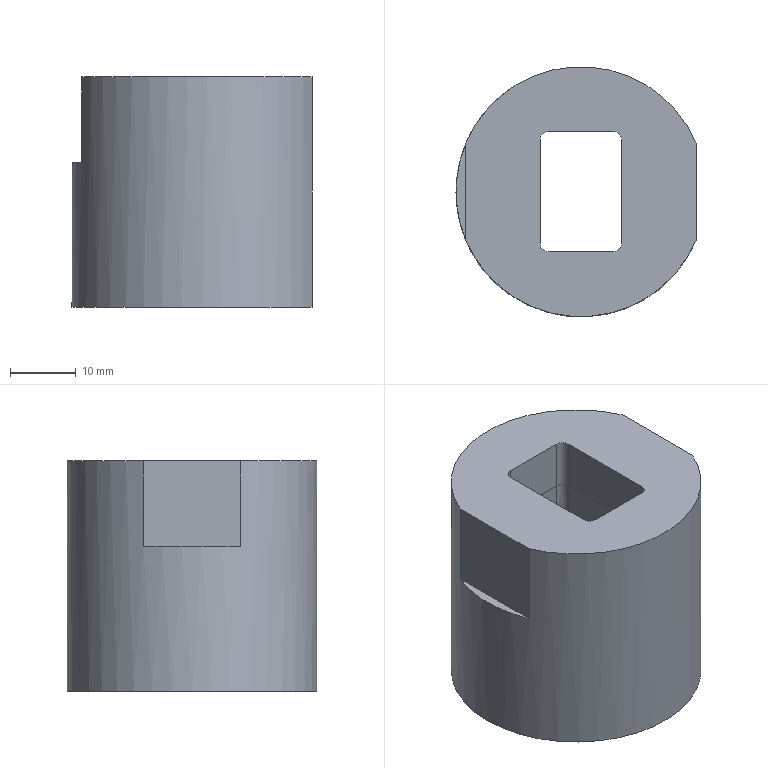Part | STEP file | lll_id4658_x_t | 1 solid | 22 faces | box 36.5 x 38 x 35 mm | volume 30517 mm3 | plane 13 | cylinder 5 | cone 4 | commonest cylinder face diameters 2.4 x4 38 x1
STEP:
#1=CARTESIAN_POINT('',(497.87,-357.252,-35.));
#2=VERTEX_POINT('',#1);
#3=CARTESIAN_POINT('',(487.87,-357.252,-35.));
#4=VERTEX_POINT('',#3);
#5=CARTESIAN_POINT('',(492.87,-357.252,-35.));
#6=DIRECTION('',(-1.,0.,0.));
#7=VECTOR('',#6,1.);
#8=LINE('',#5,#7);
#9=EDGE_CURVE('',#2,#4,#8,.T.);
#10=ORIENTED_EDGE('',*,*,#9,.F.);
#11=CARTESIAN_POINT('',(499.783,-355.34,-35.));
#12=VERTEX_POINT('',#11);
#13=CARTESIAN_POINT('',(497.87,-355.34,-35.));
#14=DIRECTION('',(0.,0.,-1.));
#15=DIRECTION('',(-1.,0.,0.));
#16=AXIS2_PLACEMENT_3D('',#13,#14,#15);
#17=CIRCLE('',#16,1.912);
#18=EDGE_CURVE('',#12,#2,#17,.T.);
#19=ORIENTED_EDGE('',*,*,#18,.F.);
#20=CARTESIAN_POINT('',(499.783,-339.5,-35.));
#21=VERTEX_POINT('',#20);
#22=CARTESIAN_POINT('',(499.783,-352.92,-35.));
#23=DIRECTION('',(0.,-1.,0.));
#24=VECTOR('',#23,1.);
#25=LINE('',#22,#24);
#26=EDGE_CURVE('',#21,#12,#25,.T.);
#27=ORIENTED_EDGE('',*,*,#26,.F.);
#28=CARTESIAN_POINT('',(497.87,-337.588,-35.));
#29=VERTEX_POINT('',#28);
#30=CARTESIAN_POINT('',(497.87,-339.5,-35.));
#31=DIRECTION('',(0.,0.,-1.));
#32=DIRECTION('',(-1.,0.,0.));
#33=AXIS2_PLACEMENT_3D('',#30,#31,#32);
#34=CIRCLE('',#33,1.912);
#35=EDGE_CURVE('',#29,#21,#34,.T.);
#36=ORIENTED_EDGE('',*,*,#35,.F.);
#37=CARTESIAN_POINT('',(487.87,-337.588,-35.));
#38=VERTEX_POINT('',#37);
#39=CARTESIAN_POINT('',(492.87,-337.588,-35.));
#40=DIRECTION('',(1.,0.,0.));
#41=VECTOR('',#40,1.);
#42=LINE('',#39,#41);
#43=EDGE_CURVE('',#38,#29,#42,.T.);
#44=ORIENTED_EDGE('',*,*,#43,.F.);
#45=CARTESIAN_POINT('',(485.958,-339.5,-35.));
#46=VERTEX_POINT('',#45);
#47=CARTESIAN_POINT('',(487.87,-339.5,-35.));
#48=DIRECTION('',(0.,0.,-1.));
#49=DIRECTION('',(-1.,0.,0.));
#50=AXIS2_PLACEMENT_3D('',#47,#48,#49);
#51=CIRCLE('',#50,1.912);
#52=EDGE_CURVE('',#46,#38,#51,.T.);
#53=ORIENTED_EDGE('',*,*,#52,.F.);
#54=CARTESIAN_POINT('',(485.958,-355.34,-35.));
#55=VERTEX_POINT('',#54);
#56=CARTESIAN_POINT('',(485.958,-352.92,-35.));
#57=DIRECTION('',(0.,1.,0.));
#58=VECTOR('',#57,1.);
#59=LINE('',#56,#58);
#60=EDGE_CURVE('',#55,#46,#59,.T.);
#61=ORIENTED_EDGE('',*,*,#60,.F.);
#62=CARTESIAN_POINT('',(487.87,-355.34,-35.));
#63=DIRECTION('',(0.,0.,-1.));
#64=DIRECTION('',(-1.,0.,0.));
#65=AXIS2_PLACEMENT_3D('',#62,#63,#64);
#66=CIRCLE('',#65,1.912);
#67=EDGE_CURVE('',#4,#55,#66,.T.);
#68=ORIENTED_EDGE('',*,*,#67,.F.);
#69=EDGE_LOOP('',(#10,#19,#27,#36,#44,#53,#61,#68));
#70=FACE_BOUND('',#69,.T.);
#71=CARTESIAN_POINT('',(510.37,-340.021,-35.));
#72=VERTEX_POINT('',#71);
#73=CARTESIAN_POINT('',(510.37,-354.819,-35.));
#74=VERTEX_POINT('',#73);
#75=CARTESIAN_POINT('',(510.37,-340.919,-35.));
#76=DIRECTION('',(0.,-1.,0.));
#77=VECTOR('',#76,1.);
#78=LINE('',#75,#77);
#79=EDGE_CURVE('',#72,#74,#78,.T.);
#80=ORIENTED_EDGE('',*,*,#79,.T.);
#81=CARTESIAN_POINT('',(492.87,-347.42,-35.));
#82=DIRECTION('',(0.,0.,1.));
#83=DIRECTION('',(1.,0.,0.));
#84=AXIS2_PLACEMENT_3D('',#81,#82,#83);
#85=CIRCLE('',#84,19.);
#86=EDGE_CURVE('',#72,#74,#85,.T.);
#87=ORIENTED_EDGE('',*,*,#86,.F.);
#88=EDGE_LOOP('',(#80,#87));
#89=FACE_BOUND('',#88,.T.);
#90=CARTESIAN_POINT('',(492.87,-352.92,-35.));
#91=DIRECTION('',(0.,0.,-1.));
#92=DIRECTION('',(0.,1.,0.));
#93=AXIS2_PLACEMENT_3D('',#90,#91,#92);
#94=PLANE('',#93);
#95=ADVANCED_FACE('',(#70,#89),#94,.T.);
#96=CARTESIAN_POINT('',(475.37,-340.021,0.));
#97=VERTEX_POINT('',#96);
#98=CARTESIAN_POINT('',(475.37,-340.021,-13.));
#99=VERTEX_POINT('',#98);
#100=CARTESIAN_POINT('',(475.37,-340.021,-15.));
#101=DIRECTION('',(0.,0.,-1.));
#102=VECTOR('',#101,1.);
#103=LINE('',#100,#102);
#104=EDGE_CURVE('',#97,#99,#103,.T.);
#105=ORIENTED_EDGE('',*,*,#104,.F.);
#106=CARTESIAN_POINT('',(510.37,-340.021,0.));
#107=VERTEX_POINT('',#106);
#108=CARTESIAN_POINT('',(492.87,-347.42,0.));
#109=DIRECTION('',(0.,0.,1.));
#110=DIRECTION('',(1.,0.,0.));
#111=AXIS2_PLACEMENT_3D('',#108,#109,#110);
#112=CIRCLE('',#111,19.);
#113=EDGE_CURVE('',#107,#97,#112,.T.);
#114=ORIENTED_EDGE('',*,*,#113,.F.);
#115=CARTESIAN_POINT('',(510.37,-340.021,0.));
#116=DIRECTION('',(0.,0.,-1.));
#117=VECTOR('',#116,1.);
#118=LINE('',#115,#117);
#119=EDGE_CURVE('',#107,#72,#118,.T.);
#120=ORIENTED_EDGE('',*,*,#119,.T.);
#121=ORIENTED_EDGE('',*,*,#86,.T.);
#122=CARTESIAN_POINT('',(510.37,-354.819,0.));
#123=VERTEX_POINT('',#122);
#124=CARTESIAN_POINT('',(510.37,-354.819,-15.));
#125=DIRECTION('',(0.,0.,1.));
#126=VECTOR('',#125,1.);
#127=LINE('',#124,#126);
#128=EDGE_CURVE('',#74,#123,#127,.T.);
#129=ORIENTED_EDGE('',*,*,#128,.T.);
#130=CARTESIAN_POINT('',(475.37,-354.819,0.));
#131=VERTEX_POINT('',#130);
#132=CARTESIAN_POINT('',(492.87,-347.42,0.));
#133=DIRECTION('',(0.,0.,1.));
#134=DIRECTION('',(1.,0.,0.));
#135=AXIS2_PLACEMENT_3D('',#132,#133,#134);
#136=CIRCLE('',#135,19.);
#137=EDGE_CURVE('',#131,#123,#136,.T.);
#138=ORIENTED_EDGE('',*,*,#137,.F.);
#139=CARTESIAN_POINT('',(475.37,-354.819,-13.));
#140=VERTEX_POINT('',#139);
#141=CARTESIAN_POINT('',(475.37,-354.819,-15.));
#142=DIRECTION('',(0.,0.,1.));
#143=VECTOR('',#142,1.);
#144=LINE('',#141,#143);
#145=EDGE_CURVE('',#140,#131,#144,.T.);
#146=ORIENTED_EDGE('',*,*,#145,.F.);
#147=CARTESIAN_POINT('',(492.87,-347.42,-13.));
#148=DIRECTION('',(0.,0.,1.));
#149=DIRECTION('',(1.,0.,0.));
#150=AXIS2_PLACEMENT_3D('',#147,#148,#149);
#151=CIRCLE('',#150,19.);
#152=EDGE_CURVE('',#99,#140,#151,.T.);
#153=ORIENTED_EDGE('',*,*,#152,.F.);
#154=EDGE_LOOP('',(#105,#114,#120,#121,#129,#138,#146,#153));
#155=FACE_OUTER_BOUND('',#154,.T.);
#156=CARTESIAN_POINT('',(492.87,-347.42,-15.));
#157=DIRECTION('',(0.,0.,-1.));
#158=DIRECTION('',(0.,-1.,0.));
#159=AXIS2_PLACEMENT_3D('',#156,#157,#158);
#160=CYLINDRICAL_SURFACE('',#159,19.);
#161=ADVANCED_FACE('',(#155),#160,.T.);
#162=CARTESIAN_POINT('',(475.37,-347.42,0.));
#163=DIRECTION('',(0.,1.,0.));
#164=VECTOR('',#163,1.);
#165=LINE('',#162,#164);
#166=EDGE_CURVE('',#131,#97,#165,.T.);
#167=ORIENTED_EDGE('',*,*,#166,.F.);
#168=ORIENTED_EDGE('',*,*,#137,.T.);
#169=CARTESIAN_POINT('',(510.37,-340.919,0.));
#170=DIRECTION('',(0.,1.,0.));
#171=VECTOR('',#170,1.);
#172=LINE('',#169,#171);
#173=EDGE_CURVE('',#123,#107,#172,.T.);
#174=ORIENTED_EDGE('',*,*,#173,.T.);
#175=ORIENTED_EDGE('',*,*,#113,.T.);
#176=EDGE_LOOP('',(#167,#168,#174,#175));
#177=FACE_BOUND('',#176,.T.);
#178=CARTESIAN_POINT('',(487.87,-356.54,0.));
#179=VERTEX_POINT('',#178);
#180=CARTESIAN_POINT('',(486.67,-355.34,0.));
#181=VERTEX_POINT('',#180);
#182=CARTESIAN_POINT('',(487.87,-355.34,0.));
#183=DIRECTION('',(0.,0.,-1.));
#184=DIRECTION('',(1.,0.,0.));
#185=AXIS2_PLACEMENT_3D('',#182,#183,#184);
#186=CIRCLE('',#185,1.2);
#187=EDGE_CURVE('',#179,#181,#186,.T.);
#188=ORIENTED_EDGE('',*,*,#187,.T.);
#189=CARTESIAN_POINT('',(486.67,-339.5,0.));
#190=VERTEX_POINT('',#189);
#191=CARTESIAN_POINT('',(486.67,-347.42,0.));
#192=DIRECTION('',(0.,1.,0.));
#193=VECTOR('',#192,1.);
#194=LINE('',#191,#193);
#195=EDGE_CURVE('',#181,#190,#194,.T.);
#196=ORIENTED_EDGE('',*,*,#195,.T.);
#197=CARTESIAN_POINT('',(487.87,-338.3,0.));
#198=VERTEX_POINT('',#197);
#199=CARTESIAN_POINT('',(487.87,-339.5,0.));
#200=DIRECTION('',(0.,0.,-1.));
#201=DIRECTION('',(1.,0.,0.));
#202=AXIS2_PLACEMENT_3D('',#199,#200,#201);
#203=CIRCLE('',#202,1.2);
#204=EDGE_CURVE('',#190,#198,#203,.T.);
#205=ORIENTED_EDGE('',*,*,#204,.T.);
#206=CARTESIAN_POINT('',(497.87,-338.3,0.));
#207=VERTEX_POINT('',#206);
#208=CARTESIAN_POINT('',(492.87,-338.3,0.));
#209=DIRECTION('',(1.,0.,0.));
#210=VECTOR('',#209,1.);
#211=LINE('',#208,#210);
#212=EDGE_CURVE('',#198,#207,#211,.T.);
#213=ORIENTED_EDGE('',*,*,#212,.T.);
#214=CARTESIAN_POINT('',(499.07,-339.5,0.));
#215=VERTEX_POINT('',#214);
#216=CARTESIAN_POINT('',(497.87,-339.5,0.));
#217=DIRECTION('',(0.,0.,-1.));
#218=DIRECTION('',(1.,0.,0.));
#219=AXIS2_PLACEMENT_3D('',#216,#217,#218);
#220=CIRCLE('',#219,1.2);
#221=EDGE_CURVE('',#207,#215,#220,.T.);
#222=ORIENTED_EDGE('',*,*,#221,.T.);
#223=CARTESIAN_POINT('',(499.07,-355.34,0.));
#224=VERTEX_POINT('',#223);
#225=CARTESIAN_POINT('',(499.07,-347.42,0.));
#226=DIRECTION('',(0.,-1.,0.));
#227=VECTOR('',#226,1.);
#228=LINE('',#225,#227);
#229=EDGE_CURVE('',#215,#224,#228,.T.);
#230=ORIENTED_EDGE('',*,*,#229,.T.);
#231=CARTESIAN_POINT('',(497.87,-356.54,0.));
#232=VERTEX_POINT('',#231);
#233=CARTESIAN_POINT('',(497.87,-355.34,0.));
#234=DIRECTION('',(0.,0.,-1.));
#235=DIRECTION('',(1.,0.,0.));
#236=AXIS2_PLACEMENT_3D('',#233,#234,#235);
#237=CIRCLE('',#236,1.2);
#238=EDGE_CURVE('',#224,#232,#237,.T.);
#239=ORIENTED_EDGE('',*,*,#238,.T.);
#240=CARTESIAN_POINT('',(492.87,-356.54,0.));
#241=DIRECTION('',(-1.,0.,0.));
#242=VECTOR('',#241,1.);
#243=LINE('',#240,#242);
#244=EDGE_CURVE('',#232,#179,#243,.T.);
#245=ORIENTED_EDGE('',*,*,#244,.T.);
#246=EDGE_LOOP('',(#188,#196,#205,#213,#222,#230,#239,#245));
#247=FACE_BOUND('',#246,.T.);
#248=CARTESIAN_POINT('',(492.87,-347.42,0.));
#249=DIRECTION('',(0.,0.,1.));
#250=DIRECTION('',(-1.,0.,0.));
#251=AXIS2_PLACEMENT_3D('',#248,#249,#250);
#252=PLANE('',#251);
#253=ADVANCED_FACE('',(#177,#247),#252,.T.);
#254=ORIENTED_EDGE('',*,*,#79,.F.);
#255=ORIENTED_EDGE('',*,*,#119,.F.);
#256=ORIENTED_EDGE('',*,*,#173,.F.);
#257=ORIENTED_EDGE('',*,*,#128,.F.);
#258=EDGE_LOOP('',(#254,#255,#256,#257));
#259=FACE_OUTER_BOUND('',#258,.T.);
#260=CARTESIAN_POINT('',(510.37,-340.919,0.));
#261=DIRECTION('',(-1.,0.,0.));
#262=DIRECTION('',(0.,0.,1.));
#263=AXIS2_PLACEMENT_3D('',#260,#261,#262);
#264=PLANE('',#263);
#265=ADVANCED_FACE('',(#259),#264,.F.);
#266=CARTESIAN_POINT('',(487.87,-356.54,-7.8));
#267=VERTEX_POINT('',#266);
#268=CARTESIAN_POINT('',(487.87,-356.54,2.5));
#269=DIRECTION('',(0.,0.,1.));
#270=VECTOR('',#269,1.);
#271=LINE('',#268,#270);
#272=EDGE_CURVE('',#267,#179,#271,.T.);
#273=ORIENTED_EDGE('',*,*,#272,.F.);
#274=CARTESIAN_POINT('',(486.67,-355.34,-7.8));
#275=VERTEX_POINT('',#274);
#276=CARTESIAN_POINT('',(487.87,-355.34,-7.8));
#277=DIRECTION('',(0.,0.,1.));
#278=DIRECTION('',(1.,0.,0.));
#279=AXIS2_PLACEMENT_3D('',#276,#277,#278);
#280=CIRCLE('',#279,1.2);
#281=EDGE_CURVE('',#275,#267,#280,.T.);
#282=ORIENTED_EDGE('',*,*,#281,.F.);
#283=CARTESIAN_POINT('',(486.67,-355.34,2.5));
#284=DIRECTION('',(0.,0.,1.));
#285=VECTOR('',#284,1.);
#286=LINE('',#283,#285);
#287=EDGE_CURVE('',#275,#181,#286,.T.);
#288=ORIENTED_EDGE('',*,*,#287,.T.);
#289=ORIENTED_EDGE('',*,*,#187,.F.);
#290=EDGE_LOOP('',(#273,#282,#288,#289));
#291=FACE_OUTER_BOUND('',#290,.T.);
#292=CARTESIAN_POINT('',(487.87,-355.34,2.5));
#293=DIRECTION('',(0.,0.,-1.));
#294=DIRECTION('',(-1.,0.,0.));
#295=AXIS2_PLACEMENT_3D('',#292,#293,#294);
#296=CYLINDRICAL_SURFACE('',#295,1.2);
#297=ADVANCED_FACE('',(#291),#296,.F.);
#298=CARTESIAN_POINT('',(497.87,-356.54,-7.8));
#299=VERTEX_POINT('',#298);
#300=CARTESIAN_POINT('',(497.87,-356.54,2.5));
#301=DIRECTION('',(0.,0.,1.));
#302=VECTOR('',#301,1.);
#303=LINE('',#300,#302);
#304=EDGE_CURVE('',#299,#232,#303,.T.);
#305=ORIENTED_EDGE('',*,*,#304,.F.);
#306=CARTESIAN_POINT('',(487.87,-356.54,-7.8));
#307=DIRECTION('',(1.,0.,0.));
#308=VECTOR('',#307,1.);
#309=LINE('',#306,#308);
#310=EDGE_CURVE('',#267,#299,#309,.T.);
#311=ORIENTED_EDGE('',*,*,#310,.F.);
#312=ORIENTED_EDGE('',*,*,#272,.T.);
#313=ORIENTED_EDGE('',*,*,#244,.F.);
#314=EDGE_LOOP('',(#305,#311,#312,#313));
#315=FACE_OUTER_BOUND('',#314,.T.);
#316=CARTESIAN_POINT('',(487.87,-356.54,2.5));
#317=DIRECTION('',(0.,-1.,0.));
#318=DIRECTION('',(0.,0.,1.));
#319=AXIS2_PLACEMENT_3D('',#316,#317,#318);
#320=PLANE('',#319);
#321=ADVANCED_FACE('',(#315),#320,.F.);
#322=CARTESIAN_POINT('',(499.07,-355.34,-7.8));
#323=VERTEX_POINT('',#322);
#324=CARTESIAN_POINT('',(499.07,-355.34,2.5));
#325=DIRECTION('',(0.,0.,1.));
#326=VECTOR('',#325,1.);
#327=LINE('',#324,#326);
#328=EDGE_CURVE('',#323,#224,#327,.T.);
#329=ORIENTED_EDGE('',*,*,#328,.F.);
#330=CARTESIAN_POINT('',(497.87,-355.34,-7.8));
#331=DIRECTION('',(0.,0.,1.));
#332=DIRECTION('',(1.,0.,0.));
#333=AXIS2_PLACEMENT_3D('',#330,#331,#332);
#334=CIRCLE('',#333,1.2);
#335=EDGE_CURVE('',#299,#323,#334,.T.);
#336=ORIENTED_EDGE('',*,*,#335,.F.);
#337=ORIENTED_EDGE('',*,*,#304,.T.);
#338=ORIENTED_EDGE('',*,*,#238,.F.);
#339=EDGE_LOOP('',(#329,#336,#337,#338));
#340=FACE_OUTER_BOUND('',#339,.T.);
#341=CARTESIAN_POINT('',(497.87,-355.34,2.5));
#342=DIRECTION('',(0.,0.,-1.));
#343=DIRECTION('',(-1.,0.,0.));
#344=AXIS2_PLACEMENT_3D('',#341,#342,#343);
#345=CYLINDRICAL_SURFACE('',#344,1.2);
#346=ADVANCED_FACE('',(#340),#345,.F.);
#347=CARTESIAN_POINT('',(499.07,-339.5,-7.8));
#348=VERTEX_POINT('',#347);
#349=CARTESIAN_POINT('',(499.07,-339.5,2.5));
#350=DIRECTION('',(0.,0.,1.));
#351=VECTOR('',#350,1.);
#352=LINE('',#349,#351);
#353=EDGE_CURVE('',#348,#215,#352,.T.);
#354=ORIENTED_EDGE('',*,*,#353,.F.);
#355=CARTESIAN_POINT('',(499.07,-355.34,-7.8));
#356=DIRECTION('',(0.,1.,0.));
#357=VECTOR('',#356,1.);
#358=LINE('',#355,#357);
#359=EDGE_CURVE('',#323,#348,#358,.T.);
#360=ORIENTED_EDGE('',*,*,#359,.F.);
#361=ORIENTED_EDGE('',*,*,#328,.T.);
#362=ORIENTED_EDGE('',*,*,#229,.F.);
#363=EDGE_LOOP('',(#354,#360,#361,#362));
#364=FACE_OUTER_BOUND('',#363,.T.);
#365=CARTESIAN_POINT('',(499.07,-355.42,2.5));
#366=DIRECTION('',(1.,0.,0.));
#367=DIRECTION('',(0.,0.,-1.));
#368=AXIS2_PLACEMENT_3D('',#365,#366,#367);
#369=PLANE('',#368);
#370=ADVANCED_FACE('',(#364),#369,.F.);
#371=CARTESIAN_POINT('',(497.87,-338.3,-7.8));
#372=VERTEX_POINT('',#371);
#373=CARTESIAN_POINT('',(497.87,-338.3,2.5));
#374=DIRECTION('',(0.,0.,1.));
#375=VECTOR('',#374,1.);
#376=LINE('',#373,#375);
#377=EDGE_CURVE('',#372,#207,#376,.T.);
#378=ORIENTED_EDGE('',*,*,#377,.F.);
#379=CARTESIAN_POINT('',(497.87,-339.5,-7.8));
#380=DIRECTION('',(0.,0.,1.));
#381=DIRECTION('',(1.,0.,0.));
#382=AXIS2_PLACEMENT_3D('',#379,#380,#381);
#383=CIRCLE('',#382,1.2);
#384=EDGE_CURVE('',#348,#372,#383,.T.);
#385=ORIENTED_EDGE('',*,*,#384,.F.);
#386=ORIENTED_EDGE('',*,*,#353,.T.);
#387=ORIENTED_EDGE('',*,*,#221,.F.);
#388=EDGE_LOOP('',(#378,#385,#386,#387));
#389=FACE_OUTER_BOUND('',#388,.T.);
#390=CARTESIAN_POINT('',(497.87,-339.5,2.5));
#391=DIRECTION('',(0.,0.,-1.));
#392=DIRECTION('',(-1.,0.,0.));
#393=AXIS2_PLACEMENT_3D('',#390,#391,#392);
#394=CYLINDRICAL_SURFACE('',#393,1.2);
#395=ADVANCED_FACE('',(#389),#394,.F.);
#396=CARTESIAN_POINT('',(487.87,-338.3,-7.8));
#397=VERTEX_POINT('',#396);
#398=CARTESIAN_POINT('',(487.87,-338.3,2.5));
#399=DIRECTION('',(0.,0.,1.));
#400=VECTOR('',#399,1.);
#401=LINE('',#398,#400);
#402=EDGE_CURVE('',#397,#198,#401,.T.);
#403=ORIENTED_EDGE('',*,*,#402,.F.);
#404=CARTESIAN_POINT('',(497.87,-338.3,-7.8));
#405=DIRECTION('',(-1.,0.,0.));
#406=VECTOR('',#405,1.);
#407=LINE('',#404,#406);
#408=EDGE_CURVE('',#372,#397,#407,.T.);
#409=ORIENTED_EDGE('',*,*,#408,.F.);
#410=ORIENTED_EDGE('',*,*,#377,.T.);
#411=ORIENTED_EDGE('',*,*,#212,.F.);
#412=EDGE_LOOP('',(#403,#409,#410,#411));
#413=FACE_OUTER_BOUND('',#412,.T.);
#414=CARTESIAN_POINT('',(497.87,-338.3,2.5));
#415=DIRECTION('',(0.,1.,0.));
#416=DIRECTION('',(0.,0.,-1.));
#417=AXIS2_PLACEMENT_3D('',#414,#415,#416);
#418=PLANE('',#417);
#419=ADVANCED_FACE('',(#413),#418,.F.);
#420=CARTESIAN_POINT('',(486.67,-339.5,-7.8));
#421=VERTEX_POINT('',#420);
#422=CARTESIAN_POINT('',(486.67,-339.5,2.5));
#423=DIRECTION('',(0.,0.,1.));
#424=VECTOR('',#423,1.);
#425=LINE('',#422,#424);
#426=EDGE_CURVE('',#421,#190,#425,.T.);
#427=ORIENTED_EDGE('',*,*,#426,.F.);
#428=CARTESIAN_POINT('',(487.87,-339.5,-7.8));
#429=DIRECTION('',(0.,0.,1.));
#430=DIRECTION('',(1.,0.,0.));
#431=AXIS2_PLACEMENT_3D('',#428,#429,#430);
#432=CIRCLE('',#431,1.2);
#433=EDGE_CURVE('',#397,#421,#432,.T.);
#434=ORIENTED_EDGE('',*,*,#433,.F.);
#435=ORIENTED_EDGE('',*,*,#402,.T.);
#436=ORIENTED_EDGE('',*,*,#204,.F.);
#437=EDGE_LOOP('',(#427,#434,#435,#436));
#438=FACE_OUTER_BOUND('',#437,.T.);
#439=CARTESIAN_POINT('',(487.87,-339.5,2.5));
#440=DIRECTION('',(0.,0.,-1.));
#441=DIRECTION('',(-1.,0.,0.));
#442=AXIS2_PLACEMENT_3D('',#439,#440,#441);
#443=CYLINDRICAL_SURFACE('',#442,1.2);
#444=ADVANCED_FACE('',(#438),#443,.F.);
#445=ORIENTED_EDGE('',*,*,#287,.F.);
#446=CARTESIAN_POINT('',(486.67,-339.5,-7.8));
#447=DIRECTION('',(0.,-1.,0.));
#448=VECTOR('',#447,1.);
#449=LINE('',#446,#448);
#450=EDGE_CURVE('',#421,#275,#449,.T.);
#451=ORIENTED_EDGE('',*,*,#450,.F.);
#452=ORIENTED_EDGE('',*,*,#426,.T.);
#453=ORIENTED_EDGE('',*,*,#195,.F.);
#454=EDGE_LOOP('',(#445,#451,#452,#453));
#455=FACE_OUTER_BOUND('',#454,.T.);
#456=CARTESIAN_POINT('',(486.67,-339.42,2.5));
#457=DIRECTION('',(-1.,0.,0.));
#458=DIRECTION('',(0.,0.,1.));
#459=AXIS2_PLACEMENT_3D('',#456,#457,#458);
#460=PLANE('',#459);
#461=ADVANCED_FACE('',(#455),#460,.F.);
#462=ORIENTED_EDGE('',*,*,#104,.T.);
#463=CARTESIAN_POINT('',(475.37,-347.42,-13.));
#464=DIRECTION('',(0.,-1.,0.));
#465=VECTOR('',#464,1.);
#466=LINE('',#463,#465);
#467=EDGE_CURVE('',#99,#140,#466,.T.);
#468=ORIENTED_EDGE('',*,*,#467,.T.);
#469=ORIENTED_EDGE('',*,*,#145,.T.);
#470=ORIENTED_EDGE('',*,*,#166,.T.);
#471=EDGE_LOOP('',(#462,#468,#469,#470));
#472=FACE_OUTER_BOUND('',#471,.T.);
#473=CARTESIAN_POINT('',(475.37,-347.42,-17.5));
#474=DIRECTION('',(1.,0.,0.));
#475=DIRECTION('',(0.,0.,-1.));
#476=AXIS2_PLACEMENT_3D('',#473,#474,#475);
#477=PLANE('',#476);
#478=ADVANCED_FACE('',(#472),#477,.F.);
#479=ORIENTED_EDGE('',*,*,#152,.T.);
#480=ORIENTED_EDGE('',*,*,#467,.F.);
#481=EDGE_LOOP('',(#479,#480));
#482=FACE_OUTER_BOUND('',#481,.T.);
#483=CARTESIAN_POINT('',(492.87,-347.42,-13.));
#484=DIRECTION('',(0.,0.,1.));
#485=DIRECTION('',(-1.,0.,0.));
#486=AXIS2_PLACEMENT_3D('',#483,#484,#485);
#487=PLANE('',#486);
#488=ADVANCED_FACE('',(#482),#487,.T.);
#489=ORIENTED_EDGE('',*,*,#9,.T.);
#490=CARTESIAN_POINT('',(487.87,-356.54,-7.8));
#491=DIRECTION('',(0.,-0.02618,-0.9997));
#492=VECTOR('',#491,1.);
#493=LINE('',#490,#492);
#494=EDGE_CURVE('',#267,#4,#493,.T.);
#495=ORIENTED_EDGE('',*,*,#494,.F.);
#496=ORIENTED_EDGE('',*,*,#310,.T.);
#497=CARTESIAN_POINT('',(497.87,-356.54,-7.8));
#498=DIRECTION('',(0.,-0.02618,-0.9997));
#499=VECTOR('',#498,1.);
#500=LINE('',#497,#499);
#501=EDGE_CURVE('',#299,#2,#500,.T.);
#502=ORIENTED_EDGE('',*,*,#501,.T.);
#503=EDGE_LOOP('',(#489,#495,#496,#502));
#504=FACE_OUTER_BOUND('',#503,.T.);
#505=CARTESIAN_POINT('',(487.87,-356.54,-7.8));
#506=DIRECTION('',(0.,0.9997,-0.02618));
#507=DIRECTION('',(0.,0.02618,0.9997));
#508=AXIS2_PLACEMENT_3D('',#505,#506,#507);
#509=PLANE('',#508);
#510=ADVANCED_FACE('',(#504),#509,.T.);
#511=ORIENTED_EDGE('',*,*,#18,.T.);
#512=ORIENTED_EDGE('',*,*,#501,.F.);
#513=ORIENTED_EDGE('',*,*,#335,.T.);
#514=CARTESIAN_POINT('',(499.07,-355.34,-7.8));
#515=DIRECTION('',(0.02618,-0.000000105,-0.9997));
#516=VECTOR('',#515,1.);
#517=LINE('',#514,#516);
#518=EDGE_CURVE('',#323,#12,#517,.T.);
#519=ORIENTED_EDGE('',*,*,#518,.T.);
#520=EDGE_LOOP('',(#511,#512,#513,#519));
#521=FACE_OUTER_BOUND('',#520,.T.);
#522=CARTESIAN_POINT('',(497.87,-355.34,-7.8));
#523=DIRECTION('',(0.,0.,-1.));
#524=DIRECTION('',(1.,0.,0.));
#525=AXIS2_PLACEMENT_3D('',#522,#523,#524);
#526=CONICAL_SURFACE('',#525,1.2,1.5);
#527=ADVANCED_FACE('',(#521),#526,.F.);
#528=ORIENTED_EDGE('',*,*,#26,.T.);
#529=ORIENTED_EDGE('',*,*,#518,.F.);
#530=ORIENTED_EDGE('',*,*,#359,.T.);
#531=CARTESIAN_POINT('',(499.07,-339.5,-7.8));
#532=DIRECTION('',(0.02618,0.,-0.9997));
#533=VECTOR('',#532,1.);
#534=LINE('',#531,#533);
#535=EDGE_CURVE('',#348,#21,#534,.T.);
#536=ORIENTED_EDGE('',*,*,#535,.T.);
#537=EDGE_LOOP('',(#528,#529,#530,#536));
#538=FACE_OUTER_BOUND('',#537,.T.);
#539=CARTESIAN_POINT('',(499.07,-355.34,-7.8));
#540=DIRECTION('',(-0.9997,0.,-0.02618));
#541=DIRECTION('',(-0.02618,0.,0.9997));
#542=AXIS2_PLACEMENT_3D('',#539,#540,#541);
#543=PLANE('',#542);
#544=ADVANCED_FACE('',(#538),#543,.T.);
#545=ORIENTED_EDGE('',*,*,#35,.T.);
#546=ORIENTED_EDGE('',*,*,#535,.F.);
#547=ORIENTED_EDGE('',*,*,#384,.T.);
#548=CARTESIAN_POINT('',(497.87,-338.3,-7.8));
#549=DIRECTION('',(0.,0.02618,-0.9997));
#550=VECTOR('',#549,1.);
#551=LINE('',#548,#550);
#552=EDGE_CURVE('',#372,#29,#551,.T.);
#553=ORIENTED_EDGE('',*,*,#552,.T.);
#554=EDGE_LOOP('',(#545,#546,#547,#553));
#555=FACE_OUTER_BOUND('',#554,.T.);
#556=CARTESIAN_POINT('',(497.87,-339.5,-7.8));
#557=DIRECTION('',(0.,0.,-1.));
#558=DIRECTION('',(1.,0.,0.));
#559=AXIS2_PLACEMENT_3D('',#556,#557,#558);
#560=CONICAL_SURFACE('',#559,1.2,1.5);
#561=ADVANCED_FACE('',(#555),#560,.F.);
#562=ORIENTED_EDGE('',*,*,#43,.T.);
#563=ORIENTED_EDGE('',*,*,#552,.F.);
#564=ORIENTED_EDGE('',*,*,#408,.T.);
#565=CARTESIAN_POINT('',(487.87,-338.3,-7.8));
#566=DIRECTION('',(0.,0.02618,-0.9997));
#567=VECTOR('',#566,1.);
#568=LINE('',#565,#567);
#569=EDGE_CURVE('',#397,#38,#568,.T.);
#570=ORIENTED_EDGE('',*,*,#569,.T.);
#571=EDGE_LOOP('',(#562,#563,#564,#570));
#572=FACE_OUTER_BOUND('',#571,.T.);
#573=CARTESIAN_POINT('',(497.87,-338.3,-7.8));
#574=DIRECTION('',(0.,-0.9997,-0.02618));
#575=DIRECTION('',(0.,0.02618,-0.9997));
#576=AXIS2_PLACEMENT_3D('',#573,#574,#575);
#577=PLANE('',#576);
#578=ADVANCED_FACE('',(#572),#577,.T.);
#579=ORIENTED_EDGE('',*,*,#52,.T.);
#580=ORIENTED_EDGE('',*,*,#569,.F.);
#581=ORIENTED_EDGE('',*,*,#433,.T.);
#582=CARTESIAN_POINT('',(486.67,-339.5,-7.8));
#583=DIRECTION('',(-0.02618,0.000000107,-0.9997));
#584=VECTOR('',#583,1.);
#585=LINE('',#582,#584);
#586=EDGE_CURVE('',#421,#46,#585,.T.);
#587=ORIENTED_EDGE('',*,*,#586,.T.);
#588=EDGE_LOOP('',(#579,#580,#581,#587));
#589=FACE_OUTER_BOUND('',#588,.T.);
#590=CARTESIAN_POINT('',(487.87,-339.5,-7.8));
#591=DIRECTION('',(0.,0.,-1.));
#592=DIRECTION('',(1.,0.,0.));
#593=AXIS2_PLACEMENT_3D('',#590,#591,#592);
#594=CONICAL_SURFACE('',#593,1.2,1.5);
#595=ADVANCED_FACE('',(#589),#594,.F.);
#596=ORIENTED_EDGE('',*,*,#60,.T.);
#597=ORIENTED_EDGE('',*,*,#586,.F.);
#598=ORIENTED_EDGE('',*,*,#450,.T.);
#599=CARTESIAN_POINT('',(486.67,-355.34,-7.8));
#600=DIRECTION('',(-0.02618,0.,-0.9997));
#601=VECTOR('',#600,1.);
#602=LINE('',#599,#601);
#603=EDGE_CURVE('',#275,#55,#602,.T.);
#604=ORIENTED_EDGE('',*,*,#603,.T.);
#605=EDGE_LOOP('',(#596,#597,#598,#604));
#606=FACE_OUTER_BOUND('',#605,.T.);
#607=CARTESIAN_POINT('',(486.67,-339.5,-7.8));
#608=DIRECTION('',(0.9997,0.,-0.02618));
#609=DIRECTION('',(-0.02618,0.,-0.9997));
#610=AXIS2_PLACEMENT_3D('',#607,#608,#609);
#611=PLANE('',#610);
#612=ADVANCED_FACE('',(#606),#611,.T.);
#613=ORIENTED_EDGE('',*,*,#67,.T.);
#614=ORIENTED_EDGE('',*,*,#603,.F.);
#615=ORIENTED_EDGE('',*,*,#281,.T.);
#616=ORIENTED_EDGE('',*,*,#494,.T.);
#617=EDGE_LOOP('',(#613,#614,#615,#616));
#618=FACE_OUTER_BOUND('',#617,.T.);
#619=CARTESIAN_POINT('',(487.87,-355.34,-7.8));
#620=DIRECTION('',(0.,0.,-1.));
#621=DIRECTION('',(1.,0.,0.));
#622=AXIS2_PLACEMENT_3D('',#619,#620,#621);
#623=CONICAL_SURFACE('',#622,1.2,1.5);
#624=ADVANCED_FACE('',(#618),#623,.F.);
#625=CLOSED_SHELL('',(#95,#161,#253,#265,#297,#321,#346,#370,#395,#419,#444,#461,#478,#488,#510,#527,#544,#561,#578,#595,#612,#624));
#626=MANIFOLD_SOLID_BREP('',#625);
#627=(LENGTH_UNIT()NAMED_UNIT(*)SI_UNIT(.MILLI.,.METRE.));
#628=UNCERTAINTY_MEASURE_WITH_UNIT(LENGTH_MEASURE(0.00002),#627,'','');
#629=(NAMED_UNIT(*)PLANE_ANGLE_UNIT()SI_UNIT($,.RADIAN.));
#630=PLANE_ANGLE_MEASURE_WITH_UNIT(PLANE_ANGLE_MEASURE(0.01745),#629);
#631=DIMENSIONAL_EXPONENTS(0.,0.,0.,0.,0.,0.,0.);
#632=(CONVERSION_BASED_UNIT('DEGREE',#630)NAMED_UNIT(#631)PLANE_ANGLE_UNIT());
#633=(NAMED_UNIT(*)SI_UNIT($,.STERADIAN.)SOLID_ANGLE_UNIT());
#634=(GEOMETRIC_REPRESENTATION_CONTEXT(3)GLOBAL_UNCERTAINTY_ASSIGNED_CONTEXT((#628))GLOBAL_UNIT_ASSIGNED_CONTEXT((#627,#632,#633))REPRESENTATION_CONTEXT('',''));
#635=ADVANCED_BREP_SHAPE_REPRESENTATION('',(#626),#634);